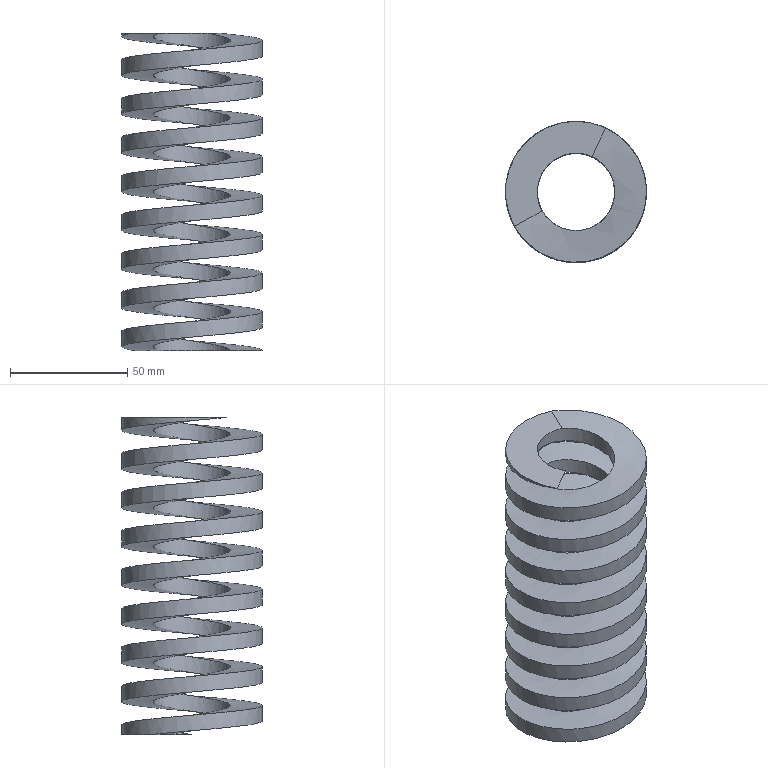Part | NX | features 模具.stp<1>[77] 2 | 1 solid | 5 faces | box 60.001 x 60 x 135.006 mm | volume 128659 mm3 | spline 2 | plane 2 | cylinder 1 | commonest cylinder face diameters 60 x1